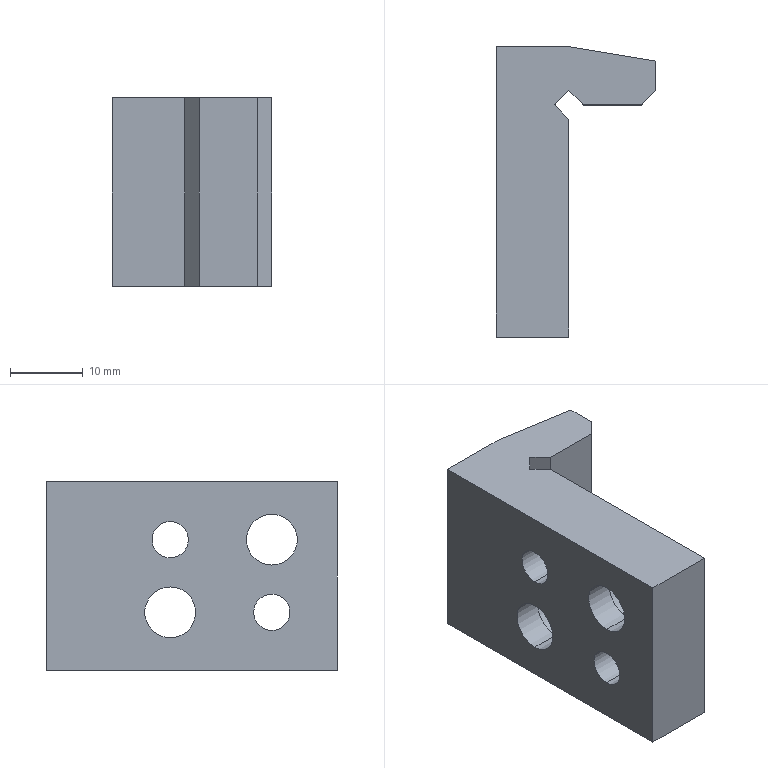Part | SolidWorks | features ICE 2, Extrusion 1 | 1 solid | 27 faces | box 22.018 x 40 x 26 mm | volume 10653 mm3 | plane 15 | cylinder 12 | commonest cylinder face diameters 5 x4 7 x4 10.5 x4
STEP:
#1=CARTESIAN_POINT('',(39.168,17.707,10.25));
#2=VERTEX_POINT('',#1);
#3=CARTESIAN_POINT('',(39.168,17.707,-0.25));
#4=VERTEX_POINT('',#3);
#5=CARTESIAN_POINT('',(39.168,17.707,5.));
#6=DIRECTION('',(1.,0.,0.));
#7=DIRECTION('',(0.,0.,-1.));
#8=AXIS2_PLACEMENT_3D('',#5,#6,#7);
#9=CIRCLE('',#8,5.25);
#10=EDGE_CURVE('',#2,#4,#9,.T.);
#11=ORIENTED_EDGE('',*,*,#10,.F.);
#12=CARTESIAN_POINT('',(45.168,17.707,10.25));
#13=VERTEX_POINT('',#12);
#14=CARTESIAN_POINT('',(39.168,17.707,10.25));
#15=DIRECTION('',(1.,0.,0.));
#16=VECTOR('',#15,1000.);
#17=LINE('',#14,#16);
#18=EDGE_CURVE('',#2,#13,#17,.T.);
#19=ORIENTED_EDGE('',*,*,#18,.T.);
#20=CARTESIAN_POINT('',(45.168,17.707,-0.25));
#21=VERTEX_POINT('',#20);
#22=CARTESIAN_POINT('',(45.168,17.707,5.));
#23=DIRECTION('',(1.,0.,0.));
#24=DIRECTION('',(0.,0.,-1.));
#25=AXIS2_PLACEMENT_3D('',#22,#23,#24);
#26=CIRCLE('',#25,5.25);
#27=EDGE_CURVE('',#13,#21,#26,.T.);
#28=ORIENTED_EDGE('',*,*,#27,.T.);
#29=CARTESIAN_POINT('',(39.168,17.707,-0.25));
#30=DIRECTION('',(1.,0.,0.));
#31=VECTOR('',#30,1000.);
#32=LINE('',#29,#31);
#33=EDGE_CURVE('',#4,#21,#32,.T.);
#34=ORIENTED_EDGE('',*,*,#33,.F.);
#35=EDGE_LOOP('',(#11,#19,#28,#34));
#36=FACE_OUTER_BOUND('',#35,.T.);
#37=CARTESIAN_POINT('',(39.168,17.707,5.));
#38=DIRECTION('',(1.,0.,0.));
#39=DIRECTION('',(0.,0.,-1.));
#40=AXIS2_PLACEMENT_3D('',#37,#38,#39);
#41=CYLINDRICAL_SURFACE('',#40,5.25);
#42=ADVANCED_FACE('',(#36),#41,.F.);
#43=CARTESIAN_POINT('',(39.168,31.707,0.25));
#44=VERTEX_POINT('',#43);
#45=CARTESIAN_POINT('',(39.168,31.707,-10.25));
#46=VERTEX_POINT('',#45);
#47=CARTESIAN_POINT('',(39.168,31.707,-5.));
#48=DIRECTION('',(1.,0.,0.));
#49=DIRECTION('',(0.,0.,-1.));
#50=AXIS2_PLACEMENT_3D('',#47,#48,#49);
#51=CIRCLE('',#50,5.25);
#52=EDGE_CURVE('',#44,#46,#51,.T.);
#53=ORIENTED_EDGE('',*,*,#52,.F.);
#54=CARTESIAN_POINT('',(45.168,31.707,0.25));
#55=VERTEX_POINT('',#54);
#56=CARTESIAN_POINT('',(39.168,31.707,0.25));
#57=DIRECTION('',(1.,0.,0.));
#58=VECTOR('',#57,1000.);
#59=LINE('',#56,#58);
#60=EDGE_CURVE('',#44,#55,#59,.T.);
#61=ORIENTED_EDGE('',*,*,#60,.T.);
#62=CARTESIAN_POINT('',(45.168,31.707,-10.25));
#63=VERTEX_POINT('',#62);
#64=CARTESIAN_POINT('',(45.168,31.707,-5.));
#65=DIRECTION('',(1.,0.,0.));
#66=DIRECTION('',(0.,0.,-1.));
#67=AXIS2_PLACEMENT_3D('',#64,#65,#66);
#68=CIRCLE('',#67,5.25);
#69=EDGE_CURVE('',#55,#63,#68,.T.);
#70=ORIENTED_EDGE('',*,*,#69,.T.);
#71=CARTESIAN_POINT('',(39.168,31.707,-10.25));
#72=DIRECTION('',(1.,0.,0.));
#73=VECTOR('',#72,1000.);
#74=LINE('',#71,#73);
#75=EDGE_CURVE('',#46,#63,#74,.T.);
#76=ORIENTED_EDGE('',*,*,#75,.F.);
#77=EDGE_LOOP('',(#53,#61,#70,#76));
#78=FACE_OUTER_BOUND('',#77,.T.);
#79=CARTESIAN_POINT('',(39.168,31.707,-5.));
#80=DIRECTION('',(1.,0.,0.));
#81=DIRECTION('',(0.,0.,-1.));
#82=AXIS2_PLACEMENT_3D('',#79,#80,#81);
#83=CYLINDRICAL_SURFACE('',#82,5.25);
#84=ADVANCED_FACE('',(#78),#83,.F.);
#85=CARTESIAN_POINT('',(35.15,31.707,7.5));
#86=VERTEX_POINT('',#85);
#87=CARTESIAN_POINT('',(35.15,31.707,2.5));
#88=VERTEX_POINT('',#87);
#89=CARTESIAN_POINT('',(35.15,31.707,5.));
#90=DIRECTION('',(1.,0.,0.));
#91=DIRECTION('',(0.,0.,-1.));
#92=AXIS2_PLACEMENT_3D('',#89,#90,#91);
#93=CIRCLE('',#92,2.5);
#94=EDGE_CURVE('',#86,#88,#93,.T.);
#95=ORIENTED_EDGE('',*,*,#94,.F.);
#96=CARTESIAN_POINT('',(45.168,31.707,7.5));
#97=VERTEX_POINT('',#96);
#98=CARTESIAN_POINT('',(19.168,31.707,7.5));
#99=DIRECTION('',(1.,0.,0.));
#100=VECTOR('',#99,1000.);
#101=LINE('',#98,#100);
#102=EDGE_CURVE('',#86,#97,#101,.T.);
#103=ORIENTED_EDGE('',*,*,#102,.T.);
#104=CARTESIAN_POINT('',(45.168,31.707,2.5));
#105=VERTEX_POINT('',#104);
#106=CARTESIAN_POINT('',(45.168,31.707,5.));
#107=DIRECTION('',(1.,0.,0.));
#108=DIRECTION('',(0.,0.,-1.));
#109=AXIS2_PLACEMENT_3D('',#106,#107,#108);
#110=CIRCLE('',#109,2.5);
#111=EDGE_CURVE('',#97,#105,#110,.T.);
#112=ORIENTED_EDGE('',*,*,#111,.T.);
#113=CARTESIAN_POINT('',(19.168,31.707,2.5));
#114=DIRECTION('',(1.,0.,0.));
#115=VECTOR('',#114,1000.);
#116=LINE('',#113,#115);
#117=EDGE_CURVE('',#88,#105,#116,.T.);
#118=ORIENTED_EDGE('',*,*,#117,.F.);
#119=EDGE_LOOP('',(#95,#103,#112,#118));
#120=FACE_OUTER_BOUND('',#119,.T.);
#121=CARTESIAN_POINT('',(19.168,31.707,5.));
#122=DIRECTION('',(1.,0.,0.));
#123=DIRECTION('',(0.,0.,-1.));
#124=AXIS2_PLACEMENT_3D('',#121,#122,#123);
#125=CYLINDRICAL_SURFACE('',#124,2.5);
#126=ADVANCED_FACE('',(#120),#125,.F.);
#127=CARTESIAN_POINT('',(35.15,17.707,-2.5));
#128=VERTEX_POINT('',#127);
#129=CARTESIAN_POINT('',(35.15,17.707,-7.5));
#130=VERTEX_POINT('',#129);
#131=CARTESIAN_POINT('',(35.15,17.707,-5.));
#132=DIRECTION('',(1.,0.,0.));
#133=DIRECTION('',(0.,0.,-1.));
#134=AXIS2_PLACEMENT_3D('',#131,#132,#133);
#135=CIRCLE('',#134,2.5);
#136=EDGE_CURVE('',#128,#130,#135,.T.);
#137=ORIENTED_EDGE('',*,*,#136,.F.);
#138=CARTESIAN_POINT('',(45.168,17.707,-2.5));
#139=VERTEX_POINT('',#138);
#140=CARTESIAN_POINT('',(19.168,17.707,-2.5));
#141=DIRECTION('',(1.,0.,0.));
#142=VECTOR('',#141,1000.);
#143=LINE('',#140,#142);
#144=EDGE_CURVE('',#128,#139,#143,.T.);
#145=ORIENTED_EDGE('',*,*,#144,.T.);
#146=CARTESIAN_POINT('',(45.168,17.707,-7.5));
#147=VERTEX_POINT('',#146);
#148=CARTESIAN_POINT('',(45.168,17.707,-5.));
#149=DIRECTION('',(1.,0.,0.));
#150=DIRECTION('',(0.,0.,-1.));
#151=AXIS2_PLACEMENT_3D('',#148,#149,#150);
#152=CIRCLE('',#151,2.5);
#153=EDGE_CURVE('',#139,#147,#152,.T.);
#154=ORIENTED_EDGE('',*,*,#153,.T.);
#155=CARTESIAN_POINT('',(19.168,17.707,-7.5));
#156=DIRECTION('',(1.,0.,0.));
#157=VECTOR('',#156,1000.);
#158=LINE('',#155,#157);
#159=EDGE_CURVE('',#130,#147,#158,.T.);
#160=ORIENTED_EDGE('',*,*,#159,.F.);
#161=EDGE_LOOP('',(#137,#145,#154,#160));
#162=FACE_OUTER_BOUND('',#161,.T.);
#163=CARTESIAN_POINT('',(19.168,17.707,-5.));
#164=DIRECTION('',(1.,0.,0.));
#165=DIRECTION('',(0.,0.,-1.));
#166=AXIS2_PLACEMENT_3D('',#163,#164,#165);
#167=CYLINDRICAL_SURFACE('',#166,2.5);
#168=ADVANCED_FACE('',(#162),#167,.F.);
#169=CARTESIAN_POINT('',(35.15,31.707,-1.5));
#170=VERTEX_POINT('',#169);
#171=CARTESIAN_POINT('',(35.15,31.707,-8.5));
#172=VERTEX_POINT('',#171);
#173=CARTESIAN_POINT('',(35.15,31.707,-5.));
#174=DIRECTION('',(1.,0.,0.));
#175=DIRECTION('',(0.,0.,-1.));
#176=AXIS2_PLACEMENT_3D('',#173,#174,#175);
#177=CIRCLE('',#176,3.5);
#178=EDGE_CURVE('',#170,#172,#177,.T.);
#179=ORIENTED_EDGE('',*,*,#178,.F.);
#180=CARTESIAN_POINT('',(39.168,31.707,-1.5));
#181=VERTEX_POINT('',#180);
#182=CARTESIAN_POINT('',(19.168,31.707,-1.5));
#183=DIRECTION('',(1.,0.,0.));
#184=VECTOR('',#183,1000.);
#185=LINE('',#182,#184);
#186=EDGE_CURVE('',#170,#181,#185,.T.);
#187=ORIENTED_EDGE('',*,*,#186,.T.);
#188=CARTESIAN_POINT('',(39.168,31.707,-8.5));
#189=VERTEX_POINT('',#188);
#190=CARTESIAN_POINT('',(39.168,31.707,-5.));
#191=DIRECTION('',(-1.,0.,0.));
#192=DIRECTION('',(0.,0.,-1.));
#193=AXIS2_PLACEMENT_3D('',#190,#191,#192);
#194=CIRCLE('',#193,3.5);
#195=EDGE_CURVE('',#189,#181,#194,.T.);
#196=ORIENTED_EDGE('',*,*,#195,.F.);
#197=CARTESIAN_POINT('',(19.168,31.707,-8.5));
#198=DIRECTION('',(1.,0.,0.));
#199=VECTOR('',#198,1000.);
#200=LINE('',#197,#199);
#201=EDGE_CURVE('',#172,#189,#200,.T.);
#202=ORIENTED_EDGE('',*,*,#201,.F.);
#203=EDGE_LOOP('',(#179,#187,#196,#202));
#204=FACE_OUTER_BOUND('',#203,.T.);
#205=CARTESIAN_POINT('',(19.168,31.707,-5.));
#206=DIRECTION('',(1.,0.,0.));
#207=DIRECTION('',(0.,0.,-1.));
#208=AXIS2_PLACEMENT_3D('',#205,#206,#207);
#209=CYLINDRICAL_SURFACE('',#208,3.5);
#210=ADVANCED_FACE('',(#204),#209,.F.);
#211=CARTESIAN_POINT('',(35.15,17.707,8.5));
#212=VERTEX_POINT('',#211);
#213=CARTESIAN_POINT('',(35.15,17.707,1.5));
#214=VERTEX_POINT('',#213);
#215=CARTESIAN_POINT('',(35.15,17.707,5.));
#216=DIRECTION('',(1.,0.,0.));
#217=DIRECTION('',(0.,0.,-1.));
#218=AXIS2_PLACEMENT_3D('',#215,#216,#217);
#219=CIRCLE('',#218,3.5);
#220=EDGE_CURVE('',#212,#214,#219,.T.);
#221=ORIENTED_EDGE('',*,*,#220,.F.);
#222=CARTESIAN_POINT('',(39.168,17.707,8.5));
#223=VERTEX_POINT('',#222);
#224=CARTESIAN_POINT('',(19.168,17.707,8.5));
#225=DIRECTION('',(1.,0.,0.));
#226=VECTOR('',#225,1000.);
#227=LINE('',#224,#226);
#228=EDGE_CURVE('',#212,#223,#227,.T.);
#229=ORIENTED_EDGE('',*,*,#228,.T.);
#230=CARTESIAN_POINT('',(39.168,17.707,1.5));
#231=VERTEX_POINT('',#230);
#232=CARTESIAN_POINT('',(39.168,17.707,5.));
#233=DIRECTION('',(-1.,0.,0.));
#234=DIRECTION('',(0.,0.,-1.));
#235=AXIS2_PLACEMENT_3D('',#232,#233,#234);
#236=CIRCLE('',#235,3.5);
#237=EDGE_CURVE('',#231,#223,#236,.T.);
#238=ORIENTED_EDGE('',*,*,#237,.F.);
#239=CARTESIAN_POINT('',(19.168,17.707,1.5));
#240=DIRECTION('',(1.,0.,0.));
#241=VECTOR('',#240,1000.);
#242=LINE('',#239,#241);
#243=EDGE_CURVE('',#214,#231,#242,.T.);
#244=ORIENTED_EDGE('',*,*,#243,.F.);
#245=EDGE_LOOP('',(#221,#229,#238,#244));
#246=FACE_OUTER_BOUND('',#245,.T.);
#247=CARTESIAN_POINT('',(19.168,17.707,5.));
#248=DIRECTION('',(1.,0.,0.));
#249=DIRECTION('',(0.,0.,-1.));
#250=AXIS2_PLACEMENT_3D('',#247,#248,#249);
#251=CYLINDRICAL_SURFACE('',#250,3.5);
#252=ADVANCED_FACE('',(#246),#251,.F.);
#253=ORIENTED_EDGE('',*,*,#228,.F.);
#254=CARTESIAN_POINT('',(35.15,17.707,5.));
#255=DIRECTION('',(1.,0.,0.));
#256=DIRECTION('',(0.,0.,-1.));
#257=AXIS2_PLACEMENT_3D('',#254,#255,#256);
#258=CIRCLE('',#257,3.5);
#259=EDGE_CURVE('',#214,#212,#258,.T.);
#260=ORIENTED_EDGE('',*,*,#259,.F.);
#261=ORIENTED_EDGE('',*,*,#243,.T.);
#262=CARTESIAN_POINT('',(39.168,17.707,5.));
#263=DIRECTION('',(-1.,0.,0.));
#264=DIRECTION('',(0.,0.,-1.));
#265=AXIS2_PLACEMENT_3D('',#262,#263,#264);
#266=CIRCLE('',#265,3.5);
#267=EDGE_CURVE('',#223,#231,#266,.T.);
#268=ORIENTED_EDGE('',*,*,#267,.F.);
#269=EDGE_LOOP('',(#253,#260,#261,#268));
#270=FACE_OUTER_BOUND('',#269,.T.);
#271=CARTESIAN_POINT('',(19.168,17.707,5.));
#272=DIRECTION('',(1.,0.,0.));
#273=DIRECTION('',(0.,0.,-1.));
#274=AXIS2_PLACEMENT_3D('',#271,#272,#273);
#275=CYLINDRICAL_SURFACE('',#274,3.5);
#276=ADVANCED_FACE('',(#270),#275,.F.);
#277=ORIENTED_EDGE('',*,*,#186,.F.);
#278=CARTESIAN_POINT('',(35.15,31.707,-5.));
#279=DIRECTION('',(1.,0.,0.));
#280=DIRECTION('',(0.,0.,-1.));
#281=AXIS2_PLACEMENT_3D('',#278,#279,#280);
#282=CIRCLE('',#281,3.5);
#283=EDGE_CURVE('',#172,#170,#282,.T.);
#284=ORIENTED_EDGE('',*,*,#283,.F.);
#285=ORIENTED_EDGE('',*,*,#201,.T.);
#286=CARTESIAN_POINT('',(39.168,31.707,-5.));
#287=DIRECTION('',(-1.,0.,0.));
#288=DIRECTION('',(0.,0.,-1.));
#289=AXIS2_PLACEMENT_3D('',#286,#287,#288);
#290=CIRCLE('',#289,3.5);
#291=EDGE_CURVE('',#181,#189,#290,.T.);
#292=ORIENTED_EDGE('',*,*,#291,.F.);
#293=EDGE_LOOP('',(#277,#284,#285,#292));
#294=FACE_OUTER_BOUND('',#293,.T.);
#295=CARTESIAN_POINT('',(19.168,31.707,-5.));
#296=DIRECTION('',(1.,0.,0.));
#297=DIRECTION('',(0.,0.,-1.));
#298=AXIS2_PLACEMENT_3D('',#295,#296,#297);
#299=CYLINDRICAL_SURFACE('',#298,3.5);
#300=ADVANCED_FACE('',(#294),#299,.F.);
#301=CARTESIAN_POINT('',(47.168,40.707,-13.));
#302=VERTEX_POINT('',#301);
#303=CARTESIAN_POINT('',(55.168,40.707,-13.));
#304=VERTEX_POINT('',#303);
#305=CARTESIAN_POINT('',(47.168,40.707,-13.));
#306=DIRECTION('',(1.,0.,0.));
#307=VECTOR('',#306,1000.);
#308=LINE('',#305,#307);
#309=EDGE_CURVE('',#302,#304,#308,.T.);
#310=ORIENTED_EDGE('',*,*,#309,.T.);
#311=CARTESIAN_POINT('',(55.168,40.707,13.));
#312=VERTEX_POINT('',#311);
#313=CARTESIAN_POINT('',(55.168,40.707,13.));
#314=DIRECTION('',(0.,0.,-1.));
#315=VECTOR('',#314,1000.);
#316=LINE('',#313,#315);
#317=EDGE_CURVE('',#312,#304,#316,.T.);
#318=ORIENTED_EDGE('',*,*,#317,.F.);
#319=CARTESIAN_POINT('',(47.168,40.707,13.));
#320=VERTEX_POINT('',#319);
#321=CARTESIAN_POINT('',(47.168,40.707,13.));
#322=DIRECTION('',(1.,0.,0.));
#323=VECTOR('',#322,1000.);
#324=LINE('',#321,#323);
#325=EDGE_CURVE('',#320,#312,#324,.T.);
#326=ORIENTED_EDGE('',*,*,#325,.F.);
#327=CARTESIAN_POINT('',(47.168,40.707,13.));
#328=DIRECTION('',(0.,0.,-1.));
#329=VECTOR('',#328,1000.);
#330=LINE('',#327,#329);
#331=EDGE_CURVE('',#320,#302,#330,.T.);
#332=ORIENTED_EDGE('',*,*,#331,.T.);
#333=EDGE_LOOP('',(#310,#318,#326,#332));
#334=FACE_OUTER_BOUND('',#333,.T.);
#335=CARTESIAN_POINT('',(47.168,40.707,13.));
#336=DIRECTION('',(0.,1.,0.));
#337=DIRECTION('',(0.,0.,1.));
#338=AXIS2_PLACEMENT_3D('',#335,#336,#337);
#339=PLANE('',#338);
#340=ADVANCED_FACE('',(#334),#339,.F.);
#341=CARTESIAN_POINT('',(57.168,42.707,-13.));
#342=VERTEX_POINT('',#341);
#343=CARTESIAN_POINT('',(55.168,40.707,-13.));
#344=DIRECTION('',(0.7071,0.7071,0.));
#345=VECTOR('',#344,1000.);
#346=LINE('',#343,#345);
#347=EDGE_CURVE('',#304,#342,#346,.T.);
#348=ORIENTED_EDGE('',*,*,#347,.T.);
#349=CARTESIAN_POINT('',(57.168,42.707,13.));
#350=VERTEX_POINT('',#349);
#351=CARTESIAN_POINT('',(57.168,42.707,13.));
#352=DIRECTION('',(0.,0.,-1.));
#353=VECTOR('',#352,1000.);
#354=LINE('',#351,#353);
#355=EDGE_CURVE('',#350,#342,#354,.T.);
#356=ORIENTED_EDGE('',*,*,#355,.F.);
#357=CARTESIAN_POINT('',(55.168,40.707,13.));
#358=DIRECTION('',(0.7071,0.7071,0.));
#359=VECTOR('',#358,1000.);
#360=LINE('',#357,#359);
#361=EDGE_CURVE('',#312,#350,#360,.T.);
#362=ORIENTED_EDGE('',*,*,#361,.F.);
#363=ORIENTED_EDGE('',*,*,#317,.T.);
#364=EDGE_LOOP('',(#348,#356,#362,#363));
#365=FACE_OUTER_BOUND('',#364,.T.);
#366=CARTESIAN_POINT('',(55.168,40.707,13.));
#367=DIRECTION('',(-0.7071,0.7071,0.));
#368=DIRECTION('',(-0.7071,-0.7071,0.));
#369=AXIS2_PLACEMENT_3D('',#366,#367,#368);
#370=PLANE('',#369);
#371=ADVANCED_FACE('',(#365),#370,.F.);
#372=CARTESIAN_POINT('',(57.168,46.707,-13.));
#373=VERTEX_POINT('',#372);
#374=CARTESIAN_POINT('',(57.168,42.707,-13.));
#375=DIRECTION('',(0.,1.,0.));
#376=VECTOR('',#375,1000.);
#377=LINE('',#374,#376);
#378=EDGE_CURVE('',#342,#373,#377,.T.);
#379=ORIENTED_EDGE('',*,*,#378,.T.);
#380=CARTESIAN_POINT('',(57.168,46.707,13.));
#381=VERTEX_POINT('',#380);
#382=CARTESIAN_POINT('',(57.168,46.707,13.));
#383=DIRECTION('',(0.,0.,-1.));
#384=VECTOR('',#383,1000.);
#385=LINE('',#382,#384);
#386=EDGE_CURVE('',#381,#373,#385,.T.);
#387=ORIENTED_EDGE('',*,*,#386,.F.);
#388=CARTESIAN_POINT('',(57.168,42.707,13.));
#389=DIRECTION('',(0.,1.,0.));
#390=VECTOR('',#389,1000.);
#391=LINE('',#388,#390);
#392=EDGE_CURVE('',#350,#381,#391,.T.);
#393=ORIENTED_EDGE('',*,*,#392,.F.);
#394=ORIENTED_EDGE('',*,*,#355,.T.);
#395=EDGE_LOOP('',(#379,#387,#393,#394));
#396=FACE_OUTER_BOUND('',#395,.T.);
#397=CARTESIAN_POINT('',(57.168,42.707,13.));
#398=DIRECTION('',(-1.,0.,0.));
#399=DIRECTION('',(0.,0.,1.));
#400=AXIS2_PLACEMENT_3D('',#397,#398,#399);
#401=PLANE('',#400);
#402=ADVANCED_FACE('',(#396),#401,.F.);
#403=CARTESIAN_POINT('',(45.168,48.707,-13.));
#404=VERTEX_POINT('',#403);
#405=CARTESIAN_POINT('',(57.168,46.707,-13.));
#406=DIRECTION('',(-0.9864,0.1644,0.));
#407=VECTOR('',#406,1000.);
#408=LINE('',#405,#407);
#409=EDGE_CURVE('',#373,#404,#408,.T.);
#410=ORIENTED_EDGE('',*,*,#409,.T.);
#411=CARTESIAN_POINT('',(45.168,48.707,13.));
#412=VERTEX_POINT('',#411);
#413=CARTESIAN_POINT('',(45.168,48.707,13.));
#414=DIRECTION('',(0.,0.,-1.));
#415=VECTOR('',#414,1000.);
#416=LINE('',#413,#415);
#417=EDGE_CURVE('',#412,#404,#416,.T.);
#418=ORIENTED_EDGE('',*,*,#417,.F.);
#419=CARTESIAN_POINT('',(57.168,46.707,13.));
#420=DIRECTION('',(-0.9864,0.1644,0.));
#421=VECTOR('',#420,1000.);
#422=LINE('',#419,#421);
#423=EDGE_CURVE('',#381,#412,#422,.T.);
#424=ORIENTED_EDGE('',*,*,#423,.F.);
#425=ORIENTED_EDGE('',*,*,#386,.T.);
#426=EDGE_LOOP('',(#410,#418,#424,#425));
#427=FACE_OUTER_BOUND('',#426,.T.);
#428=CARTESIAN_POINT('',(57.168,46.707,13.));
#429=DIRECTION('',(-0.1644,-0.9864,0.));
#430=DIRECTION('',(0.9864,-0.1644,0.));
#431=AXIS2_PLACEMENT_3D('',#428,#429,#430);
#432=PLANE('',#431);
#433=ADVANCED_FACE('',(#427),#432,.F.);
#434=CARTESIAN_POINT('',(35.15,48.707,-13.));
#435=VERTEX_POINT('',#434);
#436=CARTESIAN_POINT('',(45.168,48.707,-13.));
#437=DIRECTION('',(-1.,0.,0.));
#438=VECTOR('',#437,1000.);
#439=LINE('',#436,#438);
#440=EDGE_CURVE('',#404,#435,#439,.T.);
#441=ORIENTED_EDGE('',*,*,#440,.T.);
#442=CARTESIAN_POINT('',(35.15,48.707,13.));
#443=VERTEX_POINT('',#442);
#444=CARTESIAN_POINT('',(35.15,48.707,13.));
#445=DIRECTION('',(0.,0.,-1.));
#446=VECTOR('',#445,1000.);
#447=LINE('',#444,#446);
#448=EDGE_CURVE('',#443,#435,#447,.T.);
#449=ORIENTED_EDGE('',*,*,#448,.F.);
#450=CARTESIAN_POINT('',(45.168,48.707,13.));
#451=DIRECTION('',(-1.,0.,0.));
#452=VECTOR('',#451,1000.);
#453=LINE('',#450,#452);
#454=EDGE_CURVE('',#412,#443,#453,.T.);
#455=ORIENTED_EDGE('',*,*,#454,.F.);
#456=ORIENTED_EDGE('',*,*,#417,.T.);
#457=EDGE_LOOP('',(#441,#449,#455,#456));
#458=FACE_OUTER_BOUND('',#457,.T.);
#459=CARTESIAN_POINT('',(45.168,48.707,13.));
#460=DIRECTION('',(0.,-1.,0.));
#461=DIRECTION('',(0.,0.,-1.));
#462=AXIS2_PLACEMENT_3D('',#459,#460,#461);
#463=PLANE('',#462);
#464=ADVANCED_FACE('',(#458),#463,.F.);
#465=CARTESIAN_POINT('',(35.15,31.707,5.));
#466=DIRECTION('',(1.,0.,0.));
#467=DIRECTION('',(0.,0.,-1.));
#468=AXIS2_PLACEMENT_3D('',#465,#466,#467);
#469=CIRCLE('',#468,2.5);
#470=EDGE_CURVE('',#88,#86,#469,.T.);
#471=ORIENTED_EDGE('',*,*,#470,.T.);
#472=ORIENTED_EDGE('',*,*,#94,.T.);
#473=EDGE_LOOP('',(#471,#472));
#474=FACE_BOUND('',#473,.T.);
#475=CARTESIAN_POINT('',(35.15,17.707,-5.));
#476=DIRECTION('',(1.,0.,0.));
#477=DIRECTION('',(0.,0.,-1.));
#478=AXIS2_PLACEMENT_3D('',#475,#476,#477);
#479=CIRCLE('',#478,2.5);
#480=EDGE_CURVE('',#130,#128,#479,.T.);
#481=ORIENTED_EDGE('',*,*,#480,.T.);
#482=ORIENTED_EDGE('',*,*,#136,.T.);
#483=EDGE_LOOP('',(#481,#482));
#484=FACE_BOUND('',#483,.T.);
#485=ORIENTED_EDGE('',*,*,#283,.T.);
#486=ORIENTED_EDGE('',*,*,#178,.T.);
#487=EDGE_LOOP('',(#485,#486));
#488=FACE_BOUND('',#487,.T.);
#489=ORIENTED_EDGE('',*,*,#259,.T.);
#490=ORIENTED_EDGE('',*,*,#220,.T.);
#491=EDGE_LOOP('',(#489,#490));
#492=FACE_BOUND('',#491,.T.);
#493=CARTESIAN_POINT('',(35.15,8.707,-13.));
#494=VERTEX_POINT('',#493);
#495=CARTESIAN_POINT('',(35.15,8.707,-13.));
#496=DIRECTION('',(0.,-1.,0.));
#497=VECTOR('',#496,1000.);
#498=LINE('',#495,#497);
#499=EDGE_CURVE('',#435,#494,#498,.T.);
#500=ORIENTED_EDGE('',*,*,#499,.T.);
#501=CARTESIAN_POINT('',(35.15,8.707,13.));
#502=VERTEX_POINT('',#501);
#503=CARTESIAN_POINT('',(35.15,8.707,13.));
#504=DIRECTION('',(0.,0.,-1.));
#505=VECTOR('',#504,1000.);
#506=LINE('',#503,#505);
#507=EDGE_CURVE('',#502,#494,#506,.T.);
#508=ORIENTED_EDGE('',*,*,#507,.F.);
#509=CARTESIAN_POINT('',(35.15,14.707,13.));
#510=DIRECTION('',(0.,-1.,0.));
#511=VECTOR('',#510,1000.);
#512=LINE('',#509,#511);
#513=EDGE_CURVE('',#443,#502,#512,.T.);
#514=ORIENTED_EDGE('',*,*,#513,.F.);
#515=ORIENTED_EDGE('',*,*,#448,.T.);
#516=EDGE_LOOP('',(#500,#508,#514,#515));
#517=FACE_OUTER_BOUND('',#516,.T.);
#518=CARTESIAN_POINT('',(35.15,8.707,13.));
#519=DIRECTION('',(1.,0.,0.));
#520=DIRECTION('',(0.,0.,-1.));
#521=AXIS2_PLACEMENT_3D('',#518,#519,#520);
#522=PLANE('',#521);
#523=ADVANCED_FACE('',(#474,#484,#488,#492,#517),#522,.F.);
#524=CARTESIAN_POINT('',(45.168,8.707,-13.));
#525=VERTEX_POINT('',#524);
#526=CARTESIAN_POINT('',(35.15,8.707,-13.));
#527=DIRECTION('',(1.,0.,0.));
#528=VECTOR('',#527,1000.);
#529=LINE('',#526,#528);
#530=EDGE_CURVE('',#494,#525,#529,.T.);
#531=ORIENTED_EDGE('',*,*,#530,.T.);
#532=CARTESIAN_POINT('',(45.168,8.707,13.));
#533=VERTEX_POINT('',#532);
#534=CARTESIAN_POINT('',(45.168,8.707,13.));
#535=DIRECTION('',(0.,0.,-1.));
#536=VECTOR('',#535,1000.);
#537=LINE('',#534,#536);
#538=EDGE_CURVE('',#533,#525,#537,.T.);
#539=ORIENTED_EDGE('',*,*,#538,.F.);
#540=CARTESIAN_POINT('',(35.15,8.707,13.));
#541=DIRECTION('',(1.,0.,0.));
#542=VECTOR('',#541,1000.);
#543=LINE('',#540,#542);
#544=EDGE_CURVE('',#502,#533,#543,.T.);
#545=ORIENTED_EDGE('',*,*,#544,.F.);
#546=ORIENTED_EDGE('',*,*,#507,.T.);
#547=EDGE_LOOP('',(#531,#539,#545,#546));
#548=FACE_OUTER_BOUND('',#547,.T.);
#549=CARTESIAN_POINT('',(35.15,8.707,13.));
#550=DIRECTION('',(0.,1.,0.));
#551=DIRECTION('',(0.,0.,1.));
#552=AXIS2_PLACEMENT_3D('',#549,#550,#551);
#553=PLANE('',#552);
#554=ADVANCED_FACE('',(#548),#553,.F.);
#555=CARTESIAN_POINT('',(45.168,17.707,5.));
#556=DIRECTION('',(1.,0.,0.));
#557=DIRECTION('',(0.,0.,-1.));
#558=AXIS2_PLACEMENT_3D('',#555,#556,#557);
#559=CIRCLE('',#558,5.25);
#560=EDGE_CURVE('',#21,#13,#559,.T.);
#561=ORIENTED_EDGE('',*,*,#560,.F.);
#562=ORIENTED_EDGE('',*,*,#27,.F.);
#563=EDGE_LOOP('',(#561,#562));
#564=FACE_BOUND('',#563,.T.);
#565=CARTESIAN_POINT('',(45.168,31.707,-5.));
#566=DIRECTION('',(1.,0.,0.));
#567=DIRECTION('',(0.,0.,-1.));
#568=AXIS2_PLACEMENT_3D('',#565,#566,#567);
#569=CIRCLE('',#568,5.25);
#570=EDGE_CURVE('',#63,#55,#569,.T.);
#571=ORIENTED_EDGE('',*,*,#570,.F.);
#572=ORIENTED_EDGE('',*,*,#69,.F.);
#573=EDGE_LOOP('',(#571,#572));
#574=FACE_BOUND('',#573,.T.);
#575=CARTESIAN_POINT('',(45.168,31.707,5.));
#576=DIRECTION('',(1.,0.,0.));
#577=DIRECTION('',(0.,0.,-1.));
#578=AXIS2_PLACEMENT_3D('',#575,#576,#577);
#579=CIRCLE('',#578,2.5);
#580=EDGE_CURVE('',#105,#97,#579,.T.);
#581=ORIENTED_EDGE('',*,*,#580,.F.);
#582=ORIENTED_EDGE('',*,*,#111,.F.);
#583=EDGE_LOOP('',(#581,#582));
#584=FACE_BOUND('',#583,.T.);
#585=CARTESIAN_POINT('',(45.168,17.707,-5.));
#586=DIRECTION('',(1.,0.,0.));
#587=DIRECTION('',(0.,0.,-1.));
#588=AXIS2_PLACEMENT_3D('',#585,#586,#587);
#589=CIRCLE('',#588,2.5);
#590=EDGE_CURVE('',#147,#139,#589,.T.);
#591=ORIENTED_EDGE('',*,*,#590,.F.);
#592=ORIENTED_EDGE('',*,*,#153,.F.);
#593=EDGE_LOOP('',(#591,#592));
#594=FACE_BOUND('',#593,.T.);
#595=CARTESIAN_POINT('',(45.168,38.707,-13.));
#596=VERTEX_POINT('',#595);
#597=CARTESIAN_POINT('',(45.168,8.707,-13.));
#598=DIRECTION('',(0.,1.,0.));
#599=VECTOR('',#598,1000.);
#600=LINE('',#597,#599);
#601=EDGE_CURVE('',#525,#596,#600,.T.);
#602=ORIENTED_EDGE('',*,*,#601,.T.);
#603=CARTESIAN_POINT('',(45.168,38.707,13.));
#604=VERTEX_POINT('',#603);
#605=CARTESIAN_POINT('',(45.168,38.707,13.));
#606=DIRECTION('',(0.,0.,-1.));
#607=VECTOR('',#606,1000.);
#608=LINE('',#605,#607);
#609=EDGE_CURVE('',#604,#596,#608,.T.);
#610=ORIENTED_EDGE('',*,*,#609,.F.);
#611=CARTESIAN_POINT('',(45.168,8.707,13.));
#612=DIRECTION('',(0.,1.,0.));
#613=VECTOR('',#612,1000.);
#614=LINE('',#611,#613);
#615=EDGE_CURVE('',#533,#604,#614,.T.);
#616=ORIENTED_EDGE('',*,*,#615,.F.);
#617=ORIENTED_EDGE('',*,*,#538,.T.);
#618=EDGE_LOOP('',(#602,#610,#616,#617));
#619=FACE_OUTER_BOUND('',#618,.T.);
#620=CARTESIAN_POINT('',(45.168,8.707,13.));
#621=DIRECTION('',(-1.,0.,0.));
#622=DIRECTION('',(0.,0.,1.));
#623=AXIS2_PLACEMENT_3D('',#620,#621,#622);
#624=PLANE('',#623);
#625=ADVANCED_FACE('',(#564,#574,#584,#594,#619),#624,.F.);
#626=CARTESIAN_POINT('',(43.168,40.707,-13.));
#627=VERTEX_POINT('',#626);
#628=CARTESIAN_POINT('',(45.168,38.707,-13.));
#629=DIRECTION('',(-0.7071,0.7071,0.));
#630=VECTOR('',#629,1000.);
#631=LINE('',#628,#630);
#632=EDGE_CURVE('',#596,#627,#631,.T.);
#633=ORIENTED_EDGE('',*,*,#632,.T.);
#634=CARTESIAN_POINT('',(43.168,40.707,13.));
#635=VERTEX_POINT('',#634);
#636=CARTESIAN_POINT('',(43.168,40.707,13.));
#637=DIRECTION('',(0.,0.,-1.));
#638=VECTOR('',#637,1000.);
#639=LINE('',#636,#638);
#640=EDGE_CURVE('',#635,#627,#639,.T.);
#641=ORIENTED_EDGE('',*,*,#640,.F.);
#642=CARTESIAN_POINT('',(45.168,38.707,13.));
#643=DIRECTION('',(-0.7071,0.7071,0.));
#644=VECTOR('',#643,1000.);
#645=LINE('',#642,#644);
#646=EDGE_CURVE('',#604,#635,#645,.T.);
#647=ORIENTED_EDGE('',*,*,#646,.F.);
#648=ORIENTED_EDGE('',*,*,#609,.T.);
#649=EDGE_LOOP('',(#633,#641,#647,#648));
#650=FACE_OUTER_BOUND('',#649,.T.);
#651=CARTESIAN_POINT('',(45.168,38.707,13.));
#652=DIRECTION('',(-0.7071,-0.7071,0.));
#653=DIRECTION('',(0.7071,-0.7071,0.));
#654=AXIS2_PLACEMENT_3D('',#651,#652,#653);
#655=PLANE('',#654);
#656=ADVANCED_FACE('',(#650),#655,.F.);
#657=CARTESIAN_POINT('',(45.168,42.707,-13.));
#658=VERTEX_POINT('',#657);
#659=CARTESIAN_POINT('',(43.168,40.707,-13.));
#660=DIRECTION('',(0.7071,0.7071,0.));
#661=VECTOR('',#660,1000.);
#662=LINE('',#659,#661);
#663=EDGE_CURVE('',#627,#658,#662,.T.);
#664=ORIENTED_EDGE('',*,*,#663,.T.);
#665=CARTESIAN_POINT('',(45.168,42.707,13.));
#666=VERTEX_POINT('',#665);
#667=CARTESIAN_POINT('',(45.168,42.707,13.));
#668=DIRECTION('',(0.,0.,-1.));
#669=VECTOR('',#668,1000.);
#670=LINE('',#667,#669);
#671=EDGE_CURVE('',#666,#658,#670,.T.);
#672=ORIENTED_EDGE('',*,*,#671,.F.);
#673=CARTESIAN_POINT('',(43.168,40.707,13.));
#674=DIRECTION('',(0.7071,0.7071,0.));
#675=VECTOR('',#674,1000.);
#676=LINE('',#673,#675);
#677=EDGE_CURVE('',#635,#666,#676,.T.);
#678=ORIENTED_EDGE('',*,*,#677,.F.);
#679=ORIENTED_EDGE('',*,*,#640,.T.);
#680=EDGE_LOOP('',(#664,#672,#678,#679));
#681=FACE_OUTER_BOUND('',#680,.T.);
#682=CARTESIAN_POINT('',(43.168,40.707,13.));
#683=DIRECTION('',(-0.7071,0.7071,0.));
#684=DIRECTION('',(-0.7071,-0.7071,0.));
#685=AXIS2_PLACEMENT_3D('',#682,#683,#684);
#686=PLANE('',#685);
#687=ADVANCED_FACE('',(#681),#686,.F.);
#688=CARTESIAN_POINT('',(45.168,42.707,-13.));
#689=DIRECTION('',(0.7071,-0.7071,0.));
#690=VECTOR('',#689,1000.);
#691=LINE('',#688,#690);
#692=EDGE_CURVE('',#658,#302,#691,.T.);
#693=ORIENTED_EDGE('',*,*,#692,.T.);
#694=ORIENTED_EDGE('',*,*,#331,.F.);
#695=CARTESIAN_POINT('',(45.168,42.707,13.));
#696=DIRECTION('',(0.7071,-0.7071,0.));
#697=VECTOR('',#696,1000.);
#698=LINE('',#695,#697);
#699=EDGE_CURVE('',#666,#320,#698,.T.);
#700=ORIENTED_EDGE('',*,*,#699,.F.);
#701=ORIENTED_EDGE('',*,*,#671,.T.);
#702=EDGE_LOOP('',(#693,#694,#700,#701));
#703=FACE_OUTER_BOUND('',#702,.T.);
#704=CARTESIAN_POINT('',(45.168,42.707,13.));
#705=DIRECTION('',(0.7071,0.7071,0.));
#706=DIRECTION('',(-0.7071,0.7071,0.));
#707=AXIS2_PLACEMENT_3D('',#704,#705,#706);
#708=PLANE('',#707);
#709=ADVANCED_FACE('',(#703),#708,.F.);
#710=ORIENTED_EDGE('',*,*,#325,.T.);
#711=ORIENTED_EDGE('',*,*,#361,.T.);
#712=ORIENTED_EDGE('',*,*,#392,.T.);
#713=ORIENTED_EDGE('',*,*,#423,.T.);
#714=ORIENTED_EDGE('',*,*,#454,.T.);
#715=ORIENTED_EDGE('',*,*,#513,.T.);
#716=ORIENTED_EDGE('',*,*,#544,.T.);
#717=ORIENTED_EDGE('',*,*,#615,.T.);
#718=ORIENTED_EDGE('',*,*,#646,.T.);
#719=ORIENTED_EDGE('',*,*,#677,.T.);
#720=ORIENTED_EDGE('',*,*,#699,.T.);
#721=EDGE_LOOP('',(#710,#711,#712,#713,#714,#715,#716,#717,#718,#719,#720));
#722=FACE_OUTER_BOUND('',#721,.T.);
#723=CARTESIAN_POINT('',(57.168,40.707,13.));
#724=DIRECTION('',(0.,0.,1.));
#725=DIRECTION('',(1.,0.,0.));
#726=AXIS2_PLACEMENT_3D('',#723,#724,#725);
#727=PLANE('',#726);
#728=ADVANCED_FACE('',(#722),#727,.T.);
#729=ORIENTED_EDGE('',*,*,#309,.F.);
#730=ORIENTED_EDGE('',*,*,#692,.F.);
#731=ORIENTED_EDGE('',*,*,#663,.F.);
#732=ORIENTED_EDGE('',*,*,#632,.F.);
#733=ORIENTED_EDGE('',*,*,#601,.F.);
#734=ORIENTED_EDGE('',*,*,#530,.F.);
#735=ORIENTED_EDGE('',*,*,#499,.F.);
#736=ORIENTED_EDGE('',*,*,#440,.F.);
#737=ORIENTED_EDGE('',*,*,#409,.F.);
#738=ORIENTED_EDGE('',*,*,#378,.F.);
#739=ORIENTED_EDGE('',*,*,#347,.F.);
#740=EDGE_LOOP('',(#729,#730,#731,#732,#733,#734,#735,#736,#737,#738,#739));
#741=FACE_OUTER_BOUND('',#740,.T.);
#742=CARTESIAN_POINT('',(57.168,40.707,-13.));
#743=DIRECTION('',(0.,0.,1.));
#744=DIRECTION('',(1.,0.,0.));
#745=AXIS2_PLACEMENT_3D('',#742,#743,#744);
#746=PLANE('',#745);
#747=ADVANCED_FACE('',(#741),#746,.F.);
#748=ORIENTED_EDGE('',*,*,#144,.F.);
#749=ORIENTED_EDGE('',*,*,#480,.F.);
#750=ORIENTED_EDGE('',*,*,#159,.T.);
#751=ORIENTED_EDGE('',*,*,#590,.T.);
#752=EDGE_LOOP('',(#748,#749,#750,#751));
#753=FACE_OUTER_BOUND('',#752,.T.);
#754=CARTESIAN_POINT('',(19.168,17.707,-5.));
#755=DIRECTION('',(1.,0.,0.));
#756=DIRECTION('',(0.,0.,-1.));
#757=AXIS2_PLACEMENT_3D('',#754,#755,#756);
#758=CYLINDRICAL_SURFACE('',#757,2.5);
#759=ADVANCED_FACE('',(#753),#758,.F.);
#760=ORIENTED_EDGE('',*,*,#102,.F.);
#761=ORIENTED_EDGE('',*,*,#470,.F.);
#762=ORIENTED_EDGE('',*,*,#117,.T.);
#763=ORIENTED_EDGE('',*,*,#580,.T.);
#764=EDGE_LOOP('',(#760,#761,#762,#763));
#765=FACE_OUTER_BOUND('',#764,.T.);
#766=CARTESIAN_POINT('',(19.168,31.707,5.));
#767=DIRECTION('',(1.,0.,0.));
#768=DIRECTION('',(0.,0.,-1.));
#769=AXIS2_PLACEMENT_3D('',#766,#767,#768);
#770=CYLINDRICAL_SURFACE('',#769,2.5);
#771=ADVANCED_FACE('',(#765),#770,.F.);
#772=CARTESIAN_POINT('',(39.168,31.707,-5.));
#773=DIRECTION('',(1.,0.,0.));
#774=DIRECTION('',(0.,0.,-1.));
#775=AXIS2_PLACEMENT_3D('',#772,#773,#774);
#776=CIRCLE('',#775,5.25);
#777=EDGE_CURVE('',#46,#44,#776,.T.);
#778=ORIENTED_EDGE('',*,*,#777,.T.);
#779=ORIENTED_EDGE('',*,*,#52,.T.);
#780=EDGE_LOOP('',(#778,#779));
#781=FACE_OUTER_BOUND('',#780,.T.);
#782=ORIENTED_EDGE('',*,*,#195,.T.);
#783=ORIENTED_EDGE('',*,*,#291,.T.);
#784=EDGE_LOOP('',(#782,#783));
#785=FACE_BOUND('',#784,.T.);
#786=CARTESIAN_POINT('',(39.168,31.707,-5.));
#787=DIRECTION('',(1.,0.,0.));
#788=DIRECTION('',(0.,0.,-1.));
#789=AXIS2_PLACEMENT_3D('',#786,#787,#788);
#790=PLANE('',#789);
#791=ADVANCED_FACE('',(#781,#785),#790,.T.);
#792=ORIENTED_EDGE('',*,*,#60,.F.);
#793=ORIENTED_EDGE('',*,*,#777,.F.);
#794=ORIENTED_EDGE('',*,*,#75,.T.);
#795=ORIENTED_EDGE('',*,*,#570,.T.);
#796=EDGE_LOOP('',(#792,#793,#794,#795));
#797=FACE_OUTER_BOUND('',#796,.T.);
#798=CARTESIAN_POINT('',(39.168,31.707,-5.));
#799=DIRECTION('',(1.,0.,0.));
#800=DIRECTION('',(0.,0.,-1.));
#801=AXIS2_PLACEMENT_3D('',#798,#799,#800);
#802=CYLINDRICAL_SURFACE('',#801,5.25);
#803=ADVANCED_FACE('',(#797),#802,.F.);
#804=CARTESIAN_POINT('',(39.168,17.707,5.));
#805=DIRECTION('',(1.,0.,0.));
#806=DIRECTION('',(0.,0.,-1.));
#807=AXIS2_PLACEMENT_3D('',#804,#805,#806);
#808=CIRCLE('',#807,5.25);
#809=EDGE_CURVE('',#4,#2,#808,.T.);
#810=ORIENTED_EDGE('',*,*,#809,.T.);
#811=ORIENTED_EDGE('',*,*,#10,.T.);
#812=EDGE_LOOP('',(#810,#811));
#813=FACE_OUTER_BOUND('',#812,.T.);
#814=ORIENTED_EDGE('',*,*,#237,.T.);
#815=ORIENTED_EDGE('',*,*,#267,.T.);
#816=EDGE_LOOP('',(#814,#815));
#817=FACE_BOUND('',#816,.T.);
#818=CARTESIAN_POINT('',(39.168,17.707,5.));
#819=DIRECTION('',(1.,0.,0.));
#820=DIRECTION('',(0.,0.,-1.));
#821=AXIS2_PLACEMENT_3D('',#818,#819,#820);
#822=PLANE('',#821);
#823=ADVANCED_FACE('',(#813,#817),#822,.T.);
#824=ORIENTED_EDGE('',*,*,#18,.F.);
#825=ORIENTED_EDGE('',*,*,#809,.F.);
#826=ORIENTED_EDGE('',*,*,#33,.T.);
#827=ORIENTED_EDGE('',*,*,#560,.T.);
#828=EDGE_LOOP('',(#824,#825,#826,#827));
#829=FACE_OUTER_BOUND('',#828,.T.);
#830=CARTESIAN_POINT('',(39.168,17.707,5.));
#831=DIRECTION('',(1.,0.,0.));
#832=DIRECTION('',(0.,0.,-1.));
#833=AXIS2_PLACEMENT_3D('',#830,#831,#832);
#834=CYLINDRICAL_SURFACE('',#833,5.25);
#835=ADVANCED_FACE('',(#829),#834,.F.);
#836=CLOSED_SHELL('',(#42,#84,#126,#168,#210,#252,#276,#300,#340,#371,#402,#433,#464,#523,#554,#625,#656,#687,#709,#728,#747,#759,#771,#791,#803,#823,#835));
#837=MANIFOLD_SOLID_BREP('',#836);
#838=CARTESIAN_POINT('',(0.,0.,0.));
#839=DIRECTION('',(0.,0.,1.));
#840=DIRECTION('',(1.,0.,0.));
#841=AXIS2_PLACEMENT_3D('',#838,#839,#840);
#842=(LENGTH_UNIT()NAMED_UNIT(*)SI_UNIT(.MILLI.,.METRE.));
#843=UNCERTAINTY_MEASURE_WITH_UNIT(LENGTH_MEASURE(0.00001),#842,'','');
#844=(NAMED_UNIT(*)PLANE_ANGLE_UNIT()SI_UNIT($,.RADIAN.));
#845=(NAMED_UNIT(*)SI_UNIT($,.STERADIAN.)SOLID_ANGLE_UNIT());
#846=(GEOMETRIC_REPRESENTATION_CONTEXT(3)GLOBAL_UNCERTAINTY_ASSIGNED_CONTEXT((#843))GLOBAL_UNIT_ASSIGNED_CONTEXT((#842,#844,#845))REPRESENTATION_CONTEXT('',''));
#847=ADVANCED_BREP_SHAPE_REPRESENTATION('',(#837,#841),#846);